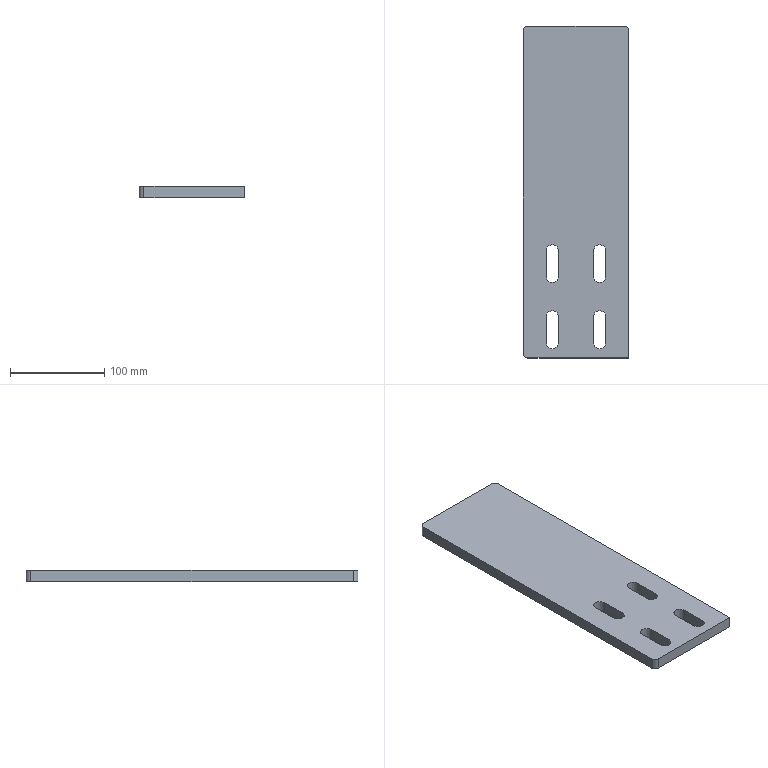Part | SolidWorks | features Extrusion 1, Fillet 1 | 1 solid | 25 faces | box 112 x 352 x 12 mm | volume 449676 mm3 | plane 14 | cylinder 11 | commonest cylinder face diameters 13 x8 10 x3
STEP:
#1=CARTESIAN_POINT('',(-56.,171.,12.));
#2=VERTEX_POINT('',#1);
#3=CARTESIAN_POINT('',(-56.,-171.,12.));
#4=VERTEX_POINT('',#3);
#5=CARTESIAN_POINT('',(-56.,176.,12.));
#6=DIRECTION('',(0.,-1.,0.));
#7=VECTOR('',#6,1000.);
#8=LINE('',#5,#7);
#9=EDGE_CURVE('',#2,#4,#8,.T.);
#10=ORIENTED_EDGE('',*,*,#9,.T.);
#11=CARTESIAN_POINT('',(-51.,-176.,12.));
#12=VERTEX_POINT('',#11);
#13=CARTESIAN_POINT('',(-51.,-171.,12.));
#14=DIRECTION('',(0.,0.,1.));
#15=DIRECTION('',(1.,0.,0.));
#16=AXIS2_PLACEMENT_3D('',#13,#14,#15);
#17=CIRCLE('',#16,5.);
#18=EDGE_CURVE('',#4,#12,#17,.T.);
#19=ORIENTED_EDGE('',*,*,#18,.T.);
#20=CARTESIAN_POINT('',(56.,-176.,12.));
#21=VERTEX_POINT('',#20);
#22=CARTESIAN_POINT('',(-56.,-176.,12.));
#23=DIRECTION('',(1.,0.,0.));
#24=VECTOR('',#23,1000.);
#25=LINE('',#22,#24);
#26=EDGE_CURVE('',#12,#21,#25,.T.);
#27=ORIENTED_EDGE('',*,*,#26,.T.);
#28=CARTESIAN_POINT('',(56.,171.,12.));
#29=VERTEX_POINT('',#28);
#30=CARTESIAN_POINT('',(56.,176.,12.));
#31=DIRECTION('',(0.,1.,0.));
#32=VECTOR('',#31,1000.);
#33=LINE('',#30,#32);
#34=EDGE_CURVE('',#21,#29,#33,.T.);
#35=ORIENTED_EDGE('',*,*,#34,.T.);
#36=CARTESIAN_POINT('',(51.,176.,12.));
#37=VERTEX_POINT('',#36);
#38=CARTESIAN_POINT('',(51.,171.,12.));
#39=DIRECTION('',(0.,0.,1.));
#40=DIRECTION('',(1.,0.,0.));
#41=AXIS2_PLACEMENT_3D('',#38,#39,#40);
#42=CIRCLE('',#41,5.);
#43=EDGE_CURVE('',#29,#37,#42,.T.);
#44=ORIENTED_EDGE('',*,*,#43,.T.);
#45=CARTESIAN_POINT('',(-51.,176.,12.));
#46=VERTEX_POINT('',#45);
#47=CARTESIAN_POINT('',(-56.,176.,12.));
#48=DIRECTION('',(-1.,0.,0.));
#49=VECTOR('',#48,1000.);
#50=LINE('',#47,#49);
#51=EDGE_CURVE('',#37,#46,#50,.T.);
#52=ORIENTED_EDGE('',*,*,#51,.T.);
#53=CARTESIAN_POINT('',(-51.,171.,12.));
#54=DIRECTION('',(0.,0.,1.));
#55=DIRECTION('',(1.,0.,0.));
#56=AXIS2_PLACEMENT_3D('',#53,#54,#55);
#57=CIRCLE('',#56,5.);
#58=EDGE_CURVE('',#46,#2,#57,.T.);
#59=ORIENTED_EDGE('',*,*,#58,.T.);
#60=EDGE_LOOP('',(#10,#19,#27,#35,#44,#52,#59));
#61=FACE_OUTER_BOUND('',#60,.T.);
#62=CARTESIAN_POINT('',(-31.5,-62.5,12.));
#63=VERTEX_POINT('',#62);
#64=CARTESIAN_POINT('',(-31.5,-89.5,12.));
#65=VERTEX_POINT('',#64);
#66=CARTESIAN_POINT('',(-31.5,-62.5,12.));
#67=DIRECTION('',(0.,-1.,0.));
#68=VECTOR('',#67,1000.);
#69=LINE('',#66,#68);
#70=EDGE_CURVE('',#63,#65,#69,.T.);
#71=ORIENTED_EDGE('',*,*,#70,.F.);
#72=CARTESIAN_POINT('',(-18.5,-62.5,12.));
#73=VERTEX_POINT('',#72);
#74=CARTESIAN_POINT('',(-25.,-62.5,12.));
#75=DIRECTION('',(0.,0.,1.));
#76=DIRECTION('',(1.,0.,0.));
#77=AXIS2_PLACEMENT_3D('',#74,#75,#76);
#78=CIRCLE('',#77,6.5);
#79=EDGE_CURVE('',#73,#63,#78,.T.);
#80=ORIENTED_EDGE('',*,*,#79,.F.);
#81=CARTESIAN_POINT('',(-18.5,-89.5,12.));
#82=VERTEX_POINT('',#81);
#83=CARTESIAN_POINT('',(-18.5,-62.5,12.));
#84=DIRECTION('',(0.,1.,0.));
#85=VECTOR('',#84,1000.);
#86=LINE('',#83,#85);
#87=EDGE_CURVE('',#82,#73,#86,.T.);
#88=ORIENTED_EDGE('',*,*,#87,.F.);
#89=CARTESIAN_POINT('',(-25.,-89.5,12.));
#90=DIRECTION('',(0.,0.,1.));
#91=DIRECTION('',(1.,0.,0.));
#92=AXIS2_PLACEMENT_3D('',#89,#90,#91);
#93=CIRCLE('',#92,6.5);
#94=EDGE_CURVE('',#65,#82,#93,.T.);
#95=ORIENTED_EDGE('',*,*,#94,.F.);
#96=EDGE_LOOP('',(#71,#80,#88,#95));
#97=FACE_BOUND('',#96,.T.);
#98=CARTESIAN_POINT('',(18.5,-62.5,12.));
#99=VERTEX_POINT('',#98);
#100=CARTESIAN_POINT('',(18.5,-89.5,12.));
#101=VERTEX_POINT('',#100);
#102=CARTESIAN_POINT('',(18.5,-62.5,12.));
#103=DIRECTION('',(0.,-1.,0.));
#104=VECTOR('',#103,1000.);
#105=LINE('',#102,#104);
#106=EDGE_CURVE('',#99,#101,#105,.T.);
#107=ORIENTED_EDGE('',*,*,#106,.F.);
#108=CARTESIAN_POINT('',(31.5,-62.5,12.));
#109=VERTEX_POINT('',#108);
#110=CARTESIAN_POINT('',(25.,-62.5,12.));
#111=DIRECTION('',(0.,0.,1.));
#112=DIRECTION('',(1.,0.,0.));
#113=AXIS2_PLACEMENT_3D('',#110,#111,#112);
#114=CIRCLE('',#113,6.5);
#115=EDGE_CURVE('',#109,#99,#114,.T.);
#116=ORIENTED_EDGE('',*,*,#115,.F.);
#117=CARTESIAN_POINT('',(31.5,-89.5,12.));
#118=VERTEX_POINT('',#117);
#119=CARTESIAN_POINT('',(31.5,-62.5,12.));
#120=DIRECTION('',(0.,1.,0.));
#121=VECTOR('',#120,1000.);
#122=LINE('',#119,#121);
#123=EDGE_CURVE('',#118,#109,#122,.T.);
#124=ORIENTED_EDGE('',*,*,#123,.F.);
#125=CARTESIAN_POINT('',(25.,-89.5,12.));
#126=DIRECTION('',(0.,0.,1.));
#127=DIRECTION('',(1.,0.,0.));
#128=AXIS2_PLACEMENT_3D('',#125,#126,#127);
#129=CIRCLE('',#128,6.5);
#130=EDGE_CURVE('',#101,#118,#129,.T.);
#131=ORIENTED_EDGE('',*,*,#130,.F.);
#132=EDGE_LOOP('',(#107,#116,#124,#131));
#133=FACE_BOUND('',#132,.T.);
#134=CARTESIAN_POINT('',(-31.5,-132.5,12.));
#135=VERTEX_POINT('',#134);
#136=CARTESIAN_POINT('',(-31.5,-159.5,12.));
#137=VERTEX_POINT('',#136);
#138=CARTESIAN_POINT('',(-31.5,-132.5,12.));
#139=DIRECTION('',(0.,-1.,0.));
#140=VECTOR('',#139,1000.);
#141=LINE('',#138,#140);
#142=EDGE_CURVE('',#135,#137,#141,.T.);
#143=ORIENTED_EDGE('',*,*,#142,.F.);
#144=CARTESIAN_POINT('',(-18.5,-132.5,12.));
#145=VERTEX_POINT('',#144);
#146=CARTESIAN_POINT('',(-25.,-132.5,12.));
#147=DIRECTION('',(0.,0.,1.));
#148=DIRECTION('',(1.,0.,0.));
#149=AXIS2_PLACEMENT_3D('',#146,#147,#148);
#150=CIRCLE('',#149,6.5);
#151=EDGE_CURVE('',#145,#135,#150,.T.);
#152=ORIENTED_EDGE('',*,*,#151,.F.);
#153=CARTESIAN_POINT('',(-18.5,-159.5,12.));
#154=VERTEX_POINT('',#153);
#155=CARTESIAN_POINT('',(-18.5,-132.5,12.));
#156=DIRECTION('',(0.,1.,0.));
#157=VECTOR('',#156,1000.);
#158=LINE('',#155,#157);
#159=EDGE_CURVE('',#154,#145,#158,.T.);
#160=ORIENTED_EDGE('',*,*,#159,.F.);
#161=CARTESIAN_POINT('',(-25.,-159.5,12.));
#162=DIRECTION('',(0.,0.,1.));
#163=DIRECTION('',(1.,0.,0.));
#164=AXIS2_PLACEMENT_3D('',#161,#162,#163);
#165=CIRCLE('',#164,6.5);
#166=EDGE_CURVE('',#137,#154,#165,.T.);
#167=ORIENTED_EDGE('',*,*,#166,.F.);
#168=EDGE_LOOP('',(#143,#152,#160,#167));
#169=FACE_BOUND('',#168,.T.);
#170=CARTESIAN_POINT('',(18.5,-132.5,12.));
#171=VERTEX_POINT('',#170);
#172=CARTESIAN_POINT('',(18.5,-159.5,12.));
#173=VERTEX_POINT('',#172);
#174=CARTESIAN_POINT('',(18.5,-132.5,12.));
#175=DIRECTION('',(0.,-1.,0.));
#176=VECTOR('',#175,1000.);
#177=LINE('',#174,#176);
#178=EDGE_CURVE('',#171,#173,#177,.T.);
#179=ORIENTED_EDGE('',*,*,#178,.F.);
#180=CARTESIAN_POINT('',(31.5,-132.5,12.));
#181=VERTEX_POINT('',#180);
#182=CARTESIAN_POINT('',(25.,-132.5,12.));
#183=DIRECTION('',(0.,0.,1.));
#184=DIRECTION('',(1.,0.,0.));
#185=AXIS2_PLACEMENT_3D('',#182,#183,#184);
#186=CIRCLE('',#185,6.5);
#187=EDGE_CURVE('',#181,#171,#186,.T.);
#188=ORIENTED_EDGE('',*,*,#187,.F.);
#189=CARTESIAN_POINT('',(31.5,-159.5,12.));
#190=VERTEX_POINT('',#189);
#191=CARTESIAN_POINT('',(31.5,-132.5,12.));
#192=DIRECTION('',(0.,1.,0.));
#193=VECTOR('',#192,1000.);
#194=LINE('',#191,#193);
#195=EDGE_CURVE('',#190,#181,#194,.T.);
#196=ORIENTED_EDGE('',*,*,#195,.F.);
#197=CARTESIAN_POINT('',(25.,-159.5,12.));
#198=DIRECTION('',(0.,0.,1.));
#199=DIRECTION('',(1.,0.,0.));
#200=AXIS2_PLACEMENT_3D('',#197,#198,#199);
#201=CIRCLE('',#200,6.5);
#202=EDGE_CURVE('',#173,#190,#201,.T.);
#203=ORIENTED_EDGE('',*,*,#202,.F.);
#204=EDGE_LOOP('',(#179,#188,#196,#203));
#205=FACE_BOUND('',#204,.T.);
#206=CARTESIAN_POINT('',(0.,0.,12.));
#207=DIRECTION('',(0.,0.,1.));
#208=DIRECTION('',(1.,0.,0.));
#209=AXIS2_PLACEMENT_3D('',#206,#207,#208);
#210=PLANE('',#209);
#211=ADVANCED_FACE('',(#61,#97,#133,#169,#205),#210,.T.);
#212=CARTESIAN_POINT('',(-18.5,-132.5,0.));
#213=VERTEX_POINT('',#212);
#214=CARTESIAN_POINT('',(-31.5,-132.5,0.));
#215=VERTEX_POINT('',#214);
#216=CARTESIAN_POINT('',(-25.,-132.5,0.));
#217=DIRECTION('',(0.,0.,1.));
#218=DIRECTION('',(1.,0.,0.));
#219=AXIS2_PLACEMENT_3D('',#216,#217,#218);
#220=CIRCLE('',#219,6.5);
#221=EDGE_CURVE('',#213,#215,#220,.T.);
#222=ORIENTED_EDGE('',*,*,#221,.T.);
#223=CARTESIAN_POINT('',(-31.5,-159.5,0.));
#224=VERTEX_POINT('',#223);
#225=CARTESIAN_POINT('',(-31.5,-132.5,0.));
#226=DIRECTION('',(0.,-1.,0.));
#227=VECTOR('',#226,1000.);
#228=LINE('',#225,#227);
#229=EDGE_CURVE('',#215,#224,#228,.T.);
#230=ORIENTED_EDGE('',*,*,#229,.T.);
#231=CARTESIAN_POINT('',(-18.5,-159.5,0.));
#232=VERTEX_POINT('',#231);
#233=CARTESIAN_POINT('',(-25.,-159.5,0.));
#234=DIRECTION('',(0.,0.,1.));
#235=DIRECTION('',(1.,0.,0.));
#236=AXIS2_PLACEMENT_3D('',#233,#234,#235);
#237=CIRCLE('',#236,6.5);
#238=EDGE_CURVE('',#224,#232,#237,.T.);
#239=ORIENTED_EDGE('',*,*,#238,.T.);
#240=CARTESIAN_POINT('',(-18.5,-132.5,0.));
#241=DIRECTION('',(0.,1.,0.));
#242=VECTOR('',#241,1000.);
#243=LINE('',#240,#242);
#244=EDGE_CURVE('',#232,#213,#243,.T.);
#245=ORIENTED_EDGE('',*,*,#244,.T.);
#246=EDGE_LOOP('',(#222,#230,#239,#245));
#247=FACE_BOUND('',#246,.T.);
#248=CARTESIAN_POINT('',(-18.5,-62.5,0.));
#249=VERTEX_POINT('',#248);
#250=CARTESIAN_POINT('',(-31.5,-62.5,0.));
#251=VERTEX_POINT('',#250);
#252=CARTESIAN_POINT('',(-25.,-62.5,0.));
#253=DIRECTION('',(0.,0.,1.));
#254=DIRECTION('',(1.,0.,0.));
#255=AXIS2_PLACEMENT_3D('',#252,#253,#254);
#256=CIRCLE('',#255,6.5);
#257=EDGE_CURVE('',#249,#251,#256,.T.);
#258=ORIENTED_EDGE('',*,*,#257,.T.);
#259=CARTESIAN_POINT('',(-31.5,-89.5,0.));
#260=VERTEX_POINT('',#259);
#261=CARTESIAN_POINT('',(-31.5,-62.5,0.));
#262=DIRECTION('',(0.,-1.,0.));
#263=VECTOR('',#262,1000.);
#264=LINE('',#261,#263);
#265=EDGE_CURVE('',#251,#260,#264,.T.);
#266=ORIENTED_EDGE('',*,*,#265,.T.);
#267=CARTESIAN_POINT('',(-18.5,-89.5,0.));
#268=VERTEX_POINT('',#267);
#269=CARTESIAN_POINT('',(-25.,-89.5,0.));
#270=DIRECTION('',(0.,0.,1.));
#271=DIRECTION('',(1.,0.,0.));
#272=AXIS2_PLACEMENT_3D('',#269,#270,#271);
#273=CIRCLE('',#272,6.5);
#274=EDGE_CURVE('',#260,#268,#273,.T.);
#275=ORIENTED_EDGE('',*,*,#274,.T.);
#276=CARTESIAN_POINT('',(-18.5,-62.5,0.));
#277=DIRECTION('',(0.,1.,0.));
#278=VECTOR('',#277,1000.);
#279=LINE('',#276,#278);
#280=EDGE_CURVE('',#268,#249,#279,.T.);
#281=ORIENTED_EDGE('',*,*,#280,.T.);
#282=EDGE_LOOP('',(#258,#266,#275,#281));
#283=FACE_BOUND('',#282,.T.);
#284=CARTESIAN_POINT('',(-51.,-176.,0.));
#285=VERTEX_POINT('',#284);
#286=CARTESIAN_POINT('',(56.,-176.,0.));
#287=VERTEX_POINT('',#286);
#288=CARTESIAN_POINT('',(-56.,-176.,0.));
#289=DIRECTION('',(1.,0.,0.));
#290=VECTOR('',#289,1000.);
#291=LINE('',#288,#290);
#292=EDGE_CURVE('',#285,#287,#291,.T.);
#293=ORIENTED_EDGE('',*,*,#292,.F.);
#294=CARTESIAN_POINT('',(-56.,-171.,0.));
#295=VERTEX_POINT('',#294);
#296=CARTESIAN_POINT('',(-51.,-171.,0.));
#297=DIRECTION('',(0.,0.,-1.));
#298=DIRECTION('',(1.,0.,0.));
#299=AXIS2_PLACEMENT_3D('',#296,#297,#298);
#300=CIRCLE('',#299,5.);
#301=EDGE_CURVE('',#285,#295,#300,.T.);
#302=ORIENTED_EDGE('',*,*,#301,.T.);
#303=CARTESIAN_POINT('',(-56.,171.,0.));
#304=VERTEX_POINT('',#303);
#305=CARTESIAN_POINT('',(-56.,176.,0.));
#306=DIRECTION('',(0.,-1.,0.));
#307=VECTOR('',#306,1000.);
#308=LINE('',#305,#307);
#309=EDGE_CURVE('',#304,#295,#308,.T.);
#310=ORIENTED_EDGE('',*,*,#309,.F.);
#311=CARTESIAN_POINT('',(-51.,176.,0.));
#312=VERTEX_POINT('',#311);
#313=CARTESIAN_POINT('',(-51.,171.,0.));
#314=DIRECTION('',(0.,0.,-1.));
#315=DIRECTION('',(1.,0.,0.));
#316=AXIS2_PLACEMENT_3D('',#313,#314,#315);
#317=CIRCLE('',#316,5.);
#318=EDGE_CURVE('',#304,#312,#317,.T.);
#319=ORIENTED_EDGE('',*,*,#318,.T.);
#320=CARTESIAN_POINT('',(51.,176.,0.));
#321=VERTEX_POINT('',#320);
#322=CARTESIAN_POINT('',(-56.,176.,0.));
#323=DIRECTION('',(-1.,0.,0.));
#324=VECTOR('',#323,1000.);
#325=LINE('',#322,#324);
#326=EDGE_CURVE('',#321,#312,#325,.T.);
#327=ORIENTED_EDGE('',*,*,#326,.F.);
#328=CARTESIAN_POINT('',(56.,171.,0.));
#329=VERTEX_POINT('',#328);
#330=CARTESIAN_POINT('',(51.,171.,0.));
#331=DIRECTION('',(0.,0.,-1.));
#332=DIRECTION('',(1.,0.,0.));
#333=AXIS2_PLACEMENT_3D('',#330,#331,#332);
#334=CIRCLE('',#333,5.);
#335=EDGE_CURVE('',#321,#329,#334,.T.);
#336=ORIENTED_EDGE('',*,*,#335,.T.);
#337=CARTESIAN_POINT('',(56.,176.,0.));
#338=DIRECTION('',(0.,1.,0.));
#339=VECTOR('',#338,1000.);
#340=LINE('',#337,#339);
#341=EDGE_CURVE('',#287,#329,#340,.T.);
#342=ORIENTED_EDGE('',*,*,#341,.F.);
#343=EDGE_LOOP('',(#293,#302,#310,#319,#327,#336,#342));
#344=FACE_OUTER_BOUND('',#343,.T.);
#345=CARTESIAN_POINT('',(31.5,-62.5,0.));
#346=VERTEX_POINT('',#345);
#347=CARTESIAN_POINT('',(18.5,-62.5,0.));
#348=VERTEX_POINT('',#347);
#349=CARTESIAN_POINT('',(25.,-62.5,0.));
#350=DIRECTION('',(0.,0.,1.));
#351=DIRECTION('',(1.,0.,0.));
#352=AXIS2_PLACEMENT_3D('',#349,#350,#351);
#353=CIRCLE('',#352,6.5);
#354=EDGE_CURVE('',#346,#348,#353,.T.);
#355=ORIENTED_EDGE('',*,*,#354,.T.);
#356=CARTESIAN_POINT('',(18.5,-89.5,0.));
#357=VERTEX_POINT('',#356);
#358=CARTESIAN_POINT('',(18.5,-62.5,0.));
#359=DIRECTION('',(0.,-1.,0.));
#360=VECTOR('',#359,1000.);
#361=LINE('',#358,#360);
#362=EDGE_CURVE('',#348,#357,#361,.T.);
#363=ORIENTED_EDGE('',*,*,#362,.T.);
#364=CARTESIAN_POINT('',(31.5,-89.5,0.));
#365=VERTEX_POINT('',#364);
#366=CARTESIAN_POINT('',(25.,-89.5,0.));
#367=DIRECTION('',(0.,0.,1.));
#368=DIRECTION('',(1.,0.,0.));
#369=AXIS2_PLACEMENT_3D('',#366,#367,#368);
#370=CIRCLE('',#369,6.5);
#371=EDGE_CURVE('',#357,#365,#370,.T.);
#372=ORIENTED_EDGE('',*,*,#371,.T.);
#373=CARTESIAN_POINT('',(31.5,-62.5,0.));
#374=DIRECTION('',(0.,1.,0.));
#375=VECTOR('',#374,1000.);
#376=LINE('',#373,#375);
#377=EDGE_CURVE('',#365,#346,#376,.T.);
#378=ORIENTED_EDGE('',*,*,#377,.T.);
#379=EDGE_LOOP('',(#355,#363,#372,#378));
#380=FACE_BOUND('',#379,.T.);
#381=CARTESIAN_POINT('',(31.5,-132.5,0.));
#382=VERTEX_POINT('',#381);
#383=CARTESIAN_POINT('',(18.5,-132.5,0.));
#384=VERTEX_POINT('',#383);
#385=CARTESIAN_POINT('',(25.,-132.5,0.));
#386=DIRECTION('',(0.,0.,1.));
#387=DIRECTION('',(1.,0.,0.));
#388=AXIS2_PLACEMENT_3D('',#385,#386,#387);
#389=CIRCLE('',#388,6.5);
#390=EDGE_CURVE('',#382,#384,#389,.T.);
#391=ORIENTED_EDGE('',*,*,#390,.T.);
#392=CARTESIAN_POINT('',(18.5,-159.5,0.));
#393=VERTEX_POINT('',#392);
#394=CARTESIAN_POINT('',(18.5,-132.5,0.));
#395=DIRECTION('',(0.,-1.,0.));
#396=VECTOR('',#395,1000.);
#397=LINE('',#394,#396);
#398=EDGE_CURVE('',#384,#393,#397,.T.);
#399=ORIENTED_EDGE('',*,*,#398,.T.);
#400=CARTESIAN_POINT('',(31.5,-159.5,0.));
#401=VERTEX_POINT('',#400);
#402=CARTESIAN_POINT('',(25.,-159.5,0.));
#403=DIRECTION('',(0.,0.,1.));
#404=DIRECTION('',(1.,0.,0.));
#405=AXIS2_PLACEMENT_3D('',#402,#403,#404);
#406=CIRCLE('',#405,6.5);
#407=EDGE_CURVE('',#393,#401,#406,.T.);
#408=ORIENTED_EDGE('',*,*,#407,.T.);
#409=CARTESIAN_POINT('',(31.5,-132.5,0.));
#410=DIRECTION('',(0.,1.,0.));
#411=VECTOR('',#410,1000.);
#412=LINE('',#409,#411);
#413=EDGE_CURVE('',#401,#382,#412,.T.);
#414=ORIENTED_EDGE('',*,*,#413,.T.);
#415=EDGE_LOOP('',(#391,#399,#408,#414));
#416=FACE_BOUND('',#415,.T.);
#417=CARTESIAN_POINT('',(0.,0.,0.));
#418=DIRECTION('',(0.,0.,1.));
#419=DIRECTION('',(1.,0.,0.));
#420=AXIS2_PLACEMENT_3D('',#417,#418,#419);
#421=PLANE('',#420);
#422=ADVANCED_FACE('',(#247,#283,#344,#380,#416),#421,.F.);
#423=ORIENTED_EDGE('',*,*,#341,.T.);
#424=CARTESIAN_POINT('',(56.,171.,12.));
#425=DIRECTION('',(0.,0.,1.));
#426=VECTOR('',#425,1000.);
#427=LINE('',#424,#426);
#428=EDGE_CURVE('',#329,#29,#427,.T.);
#429=ORIENTED_EDGE('',*,*,#428,.T.);
#430=ORIENTED_EDGE('',*,*,#34,.F.);
#431=CARTESIAN_POINT('',(56.,-176.,12.));
#432=DIRECTION('',(0.,0.,-1.));
#433=VECTOR('',#432,1000.);
#434=LINE('',#431,#433);
#435=EDGE_CURVE('',#21,#287,#434,.T.);
#436=ORIENTED_EDGE('',*,*,#435,.T.);
#437=EDGE_LOOP('',(#423,#429,#430,#436));
#438=FACE_OUTER_BOUND('',#437,.T.);
#439=CARTESIAN_POINT('',(56.,176.,12.));
#440=DIRECTION('',(-1.,0.,0.));
#441=DIRECTION('',(0.,-1.,0.));
#442=AXIS2_PLACEMENT_3D('',#439,#440,#441);
#443=PLANE('',#442);
#444=ADVANCED_FACE('',(#438),#443,.F.);
#445=ORIENTED_EDGE('',*,*,#51,.F.);
#446=CARTESIAN_POINT('',(51.,176.,12.));
#447=DIRECTION('',(0.,0.,-1.));
#448=VECTOR('',#447,1000.);
#449=LINE('',#446,#448);
#450=EDGE_CURVE('',#37,#321,#449,.T.);
#451=ORIENTED_EDGE('',*,*,#450,.T.);
#452=ORIENTED_EDGE('',*,*,#326,.T.);
#453=CARTESIAN_POINT('',(-51.,176.,12.));
#454=DIRECTION('',(0.,0.,1.));
#455=VECTOR('',#454,1000.);
#456=LINE('',#453,#455);
#457=EDGE_CURVE('',#312,#46,#456,.T.);
#458=ORIENTED_EDGE('',*,*,#457,.T.);
#459=EDGE_LOOP('',(#445,#451,#452,#458));
#460=FACE_OUTER_BOUND('',#459,.T.);
#461=CARTESIAN_POINT('',(-56.,176.,12.));
#462=DIRECTION('',(0.,-1.,0.));
#463=DIRECTION('',(0.,0.,-1.));
#464=AXIS2_PLACEMENT_3D('',#461,#462,#463);
#465=PLANE('',#464);
#466=ADVANCED_FACE('',(#460),#465,.F.);
#467=ORIENTED_EDGE('',*,*,#309,.T.);
#468=CARTESIAN_POINT('',(-56.,-171.,12.));
#469=DIRECTION('',(0.,0.,1.));
#470=VECTOR('',#469,1000.);
#471=LINE('',#468,#470);
#472=EDGE_CURVE('',#295,#4,#471,.T.);
#473=ORIENTED_EDGE('',*,*,#472,.T.);
#474=ORIENTED_EDGE('',*,*,#9,.F.);
#475=CARTESIAN_POINT('',(-56.,171.,12.));
#476=DIRECTION('',(0.,0.,-1.));
#477=VECTOR('',#476,1000.);
#478=LINE('',#475,#477);
#479=EDGE_CURVE('',#2,#304,#478,.T.);
#480=ORIENTED_EDGE('',*,*,#479,.T.);
#481=EDGE_LOOP('',(#467,#473,#474,#480));
#482=FACE_OUTER_BOUND('',#481,.T.);
#483=CARTESIAN_POINT('',(-56.,176.,12.));
#484=DIRECTION('',(1.,0.,0.));
#485=DIRECTION('',(0.,1.,0.));
#486=AXIS2_PLACEMENT_3D('',#483,#484,#485);
#487=PLANE('',#486);
#488=ADVANCED_FACE('',(#482),#487,.F.);
#489=ORIENTED_EDGE('',*,*,#26,.F.);
#490=CARTESIAN_POINT('',(-51.,-176.,12.));
#491=DIRECTION('',(0.,0.,-1.));
#492=VECTOR('',#491,1000.);
#493=LINE('',#490,#492);
#494=EDGE_CURVE('',#12,#285,#493,.T.);
#495=ORIENTED_EDGE('',*,*,#494,.T.);
#496=ORIENTED_EDGE('',*,*,#292,.T.);
#497=ORIENTED_EDGE('',*,*,#435,.F.);
#498=EDGE_LOOP('',(#489,#495,#496,#497));
#499=FACE_OUTER_BOUND('',#498,.T.);
#500=CARTESIAN_POINT('',(-56.,-176.,12.));
#501=DIRECTION('',(0.,1.,0.));
#502=DIRECTION('',(0.,0.,1.));
#503=AXIS2_PLACEMENT_3D('',#500,#501,#502);
#504=PLANE('',#503);
#505=ADVANCED_FACE('',(#499),#504,.F.);
#506=ORIENTED_EDGE('',*,*,#257,.F.);
#507=CARTESIAN_POINT('',(-18.5,-62.5,12.));
#508=DIRECTION('',(0.,0.,-1.));
#509=VECTOR('',#508,1000.);
#510=LINE('',#507,#509);
#511=EDGE_CURVE('',#73,#249,#510,.T.);
#512=ORIENTED_EDGE('',*,*,#511,.F.);
#513=ORIENTED_EDGE('',*,*,#79,.T.);
#514=CARTESIAN_POINT('',(-31.5,-62.5,12.));
#515=DIRECTION('',(0.,0.,-1.));
#516=VECTOR('',#515,1000.);
#517=LINE('',#514,#516);
#518=EDGE_CURVE('',#63,#251,#517,.T.);
#519=ORIENTED_EDGE('',*,*,#518,.T.);
#520=EDGE_LOOP('',(#506,#512,#513,#519));
#521=FACE_OUTER_BOUND('',#520,.T.);
#522=CARTESIAN_POINT('',(-25.,-62.5,12.));
#523=DIRECTION('',(0.,0.,-1.));
#524=DIRECTION('',(-1.,0.,0.));
#525=AXIS2_PLACEMENT_3D('',#522,#523,#524);
#526=CYLINDRICAL_SURFACE('',#525,6.5);
#527=ADVANCED_FACE('',(#521),#526,.F.);
#528=ORIENTED_EDGE('',*,*,#265,.F.);
#529=ORIENTED_EDGE('',*,*,#518,.F.);
#530=ORIENTED_EDGE('',*,*,#70,.T.);
#531=CARTESIAN_POINT('',(-31.5,-89.5,12.));
#532=DIRECTION('',(0.,0.,-1.));
#533=VECTOR('',#532,1000.);
#534=LINE('',#531,#533);
#535=EDGE_CURVE('',#65,#260,#534,.T.);
#536=ORIENTED_EDGE('',*,*,#535,.T.);
#537=EDGE_LOOP('',(#528,#529,#530,#536));
#538=FACE_OUTER_BOUND('',#537,.T.);
#539=CARTESIAN_POINT('',(-31.5,-62.5,12.));
#540=DIRECTION('',(1.,0.,0.));
#541=DIRECTION('',(0.,1.,0.));
#542=AXIS2_PLACEMENT_3D('',#539,#540,#541);
#543=PLANE('',#542);
#544=ADVANCED_FACE('',(#538),#543,.T.);
#545=ORIENTED_EDGE('',*,*,#274,.F.);
#546=ORIENTED_EDGE('',*,*,#535,.F.);
#547=ORIENTED_EDGE('',*,*,#94,.T.);
#548=CARTESIAN_POINT('',(-18.5,-89.5,12.));
#549=DIRECTION('',(0.,0.,-1.));
#550=VECTOR('',#549,1000.);
#551=LINE('',#548,#550);
#552=EDGE_CURVE('',#82,#268,#551,.T.);
#553=ORIENTED_EDGE('',*,*,#552,.T.);
#554=EDGE_LOOP('',(#545,#546,#547,#553));
#555=FACE_OUTER_BOUND('',#554,.T.);
#556=CARTESIAN_POINT('',(-25.,-89.5,12.));
#557=DIRECTION('',(0.,0.,-1.));
#558=DIRECTION('',(-1.,0.,0.));
#559=AXIS2_PLACEMENT_3D('',#556,#557,#558);
#560=CYLINDRICAL_SURFACE('',#559,6.5);
#561=ADVANCED_FACE('',(#555),#560,.F.);
#562=ORIENTED_EDGE('',*,*,#280,.F.);
#563=ORIENTED_EDGE('',*,*,#552,.F.);
#564=ORIENTED_EDGE('',*,*,#87,.T.);
#565=ORIENTED_EDGE('',*,*,#511,.T.);
#566=EDGE_LOOP('',(#562,#563,#564,#565));
#567=FACE_OUTER_BOUND('',#566,.T.);
#568=CARTESIAN_POINT('',(-18.5,-62.5,12.));
#569=DIRECTION('',(-1.,0.,0.));
#570=DIRECTION('',(0.,0.,1.));
#571=AXIS2_PLACEMENT_3D('',#568,#569,#570);
#572=PLANE('',#571);
#573=ADVANCED_FACE('',(#567),#572,.T.);
#574=ORIENTED_EDGE('',*,*,#354,.F.);
#575=CARTESIAN_POINT('',(31.5,-62.5,12.));
#576=DIRECTION('',(0.,0.,-1.));
#577=VECTOR('',#576,1000.);
#578=LINE('',#575,#577);
#579=EDGE_CURVE('',#109,#346,#578,.T.);
#580=ORIENTED_EDGE('',*,*,#579,.F.);
#581=ORIENTED_EDGE('',*,*,#115,.T.);
#582=CARTESIAN_POINT('',(18.5,-62.5,12.));
#583=DIRECTION('',(0.,0.,-1.));
#584=VECTOR('',#583,1000.);
#585=LINE('',#582,#584);
#586=EDGE_CURVE('',#99,#348,#585,.T.);
#587=ORIENTED_EDGE('',*,*,#586,.T.);
#588=EDGE_LOOP('',(#574,#580,#581,#587));
#589=FACE_OUTER_BOUND('',#588,.T.);
#590=CARTESIAN_POINT('',(25.,-62.5,12.));
#591=DIRECTION('',(0.,0.,-1.));
#592=DIRECTION('',(-1.,0.,0.));
#593=AXIS2_PLACEMENT_3D('',#590,#591,#592);
#594=CYLINDRICAL_SURFACE('',#593,6.5);
#595=ADVANCED_FACE('',(#589),#594,.F.);
#596=ORIENTED_EDGE('',*,*,#362,.F.);
#597=ORIENTED_EDGE('',*,*,#586,.F.);
#598=ORIENTED_EDGE('',*,*,#106,.T.);
#599=CARTESIAN_POINT('',(18.5,-89.5,12.));
#600=DIRECTION('',(0.,0.,-1.));
#601=VECTOR('',#600,1000.);
#602=LINE('',#599,#601);
#603=EDGE_CURVE('',#101,#357,#602,.T.);
#604=ORIENTED_EDGE('',*,*,#603,.T.);
#605=EDGE_LOOP('',(#596,#597,#598,#604));
#606=FACE_OUTER_BOUND('',#605,.T.);
#607=CARTESIAN_POINT('',(18.5,-62.5,12.));
#608=DIRECTION('',(1.,0.,0.));
#609=DIRECTION('',(0.,0.,-1.));
#610=AXIS2_PLACEMENT_3D('',#607,#608,#609);
#611=PLANE('',#610);
#612=ADVANCED_FACE('',(#606),#611,.T.);
#613=ORIENTED_EDGE('',*,*,#371,.F.);
#614=ORIENTED_EDGE('',*,*,#603,.F.);
#615=ORIENTED_EDGE('',*,*,#130,.T.);
#616=CARTESIAN_POINT('',(31.5,-89.5,12.));
#617=DIRECTION('',(0.,0.,-1.));
#618=VECTOR('',#617,1000.);
#619=LINE('',#616,#618);
#620=EDGE_CURVE('',#118,#365,#619,.T.);
#621=ORIENTED_EDGE('',*,*,#620,.T.);
#622=EDGE_LOOP('',(#613,#614,#615,#621));
#623=FACE_OUTER_BOUND('',#622,.T.);
#624=CARTESIAN_POINT('',(25.,-89.5,12.));
#625=DIRECTION('',(0.,0.,-1.));
#626=DIRECTION('',(-1.,0.,0.));
#627=AXIS2_PLACEMENT_3D('',#624,#625,#626);
#628=CYLINDRICAL_SURFACE('',#627,6.5);
#629=ADVANCED_FACE('',(#623),#628,.F.);
#630=ORIENTED_EDGE('',*,*,#377,.F.);
#631=ORIENTED_EDGE('',*,*,#620,.F.);
#632=ORIENTED_EDGE('',*,*,#123,.T.);
#633=ORIENTED_EDGE('',*,*,#579,.T.);
#634=EDGE_LOOP('',(#630,#631,#632,#633));
#635=FACE_OUTER_BOUND('',#634,.T.);
#636=CARTESIAN_POINT('',(31.5,-62.5,12.));
#637=DIRECTION('',(-1.,0.,0.));
#638=DIRECTION('',(0.,0.,1.));
#639=AXIS2_PLACEMENT_3D('',#636,#637,#638);
#640=PLANE('',#639);
#641=ADVANCED_FACE('',(#635),#640,.T.);
#642=ORIENTED_EDGE('',*,*,#221,.F.);
#643=CARTESIAN_POINT('',(-18.5,-132.5,12.));
#644=DIRECTION('',(0.,0.,-1.));
#645=VECTOR('',#644,1000.);
#646=LINE('',#643,#645);
#647=EDGE_CURVE('',#145,#213,#646,.T.);
#648=ORIENTED_EDGE('',*,*,#647,.F.);
#649=ORIENTED_EDGE('',*,*,#151,.T.);
#650=CARTESIAN_POINT('',(-31.5,-132.5,12.));
#651=DIRECTION('',(0.,0.,-1.));
#652=VECTOR('',#651,1000.);
#653=LINE('',#650,#652);
#654=EDGE_CURVE('',#135,#215,#653,.T.);
#655=ORIENTED_EDGE('',*,*,#654,.T.);
#656=EDGE_LOOP('',(#642,#648,#649,#655));
#657=FACE_OUTER_BOUND('',#656,.T.);
#658=CARTESIAN_POINT('',(-25.,-132.5,12.));
#659=DIRECTION('',(0.,0.,-1.));
#660=DIRECTION('',(-1.,0.,0.));
#661=AXIS2_PLACEMENT_3D('',#658,#659,#660);
#662=CYLINDRICAL_SURFACE('',#661,6.5);
#663=ADVANCED_FACE('',(#657),#662,.F.);
#664=ORIENTED_EDGE('',*,*,#229,.F.);
#665=ORIENTED_EDGE('',*,*,#654,.F.);
#666=ORIENTED_EDGE('',*,*,#142,.T.);
#667=CARTESIAN_POINT('',(-31.5,-159.5,12.));
#668=DIRECTION('',(0.,0.,-1.));
#669=VECTOR('',#668,1000.);
#670=LINE('',#667,#669);
#671=EDGE_CURVE('',#137,#224,#670,.T.);
#672=ORIENTED_EDGE('',*,*,#671,.T.);
#673=EDGE_LOOP('',(#664,#665,#666,#672));
#674=FACE_OUTER_BOUND('',#673,.T.);
#675=CARTESIAN_POINT('',(-31.5,-132.5,12.));
#676=DIRECTION('',(1.,0.,0.));
#677=DIRECTION('',(0.,1.,0.));
#678=AXIS2_PLACEMENT_3D('',#675,#676,#677);
#679=PLANE('',#678);
#680=ADVANCED_FACE('',(#674),#679,.T.);
#681=ORIENTED_EDGE('',*,*,#238,.F.);
#682=ORIENTED_EDGE('',*,*,#671,.F.);
#683=ORIENTED_EDGE('',*,*,#166,.T.);
#684=CARTESIAN_POINT('',(-18.5,-159.5,12.));
#685=DIRECTION('',(0.,0.,-1.));
#686=VECTOR('',#685,1000.);
#687=LINE('',#684,#686);
#688=EDGE_CURVE('',#154,#232,#687,.T.);
#689=ORIENTED_EDGE('',*,*,#688,.T.);
#690=EDGE_LOOP('',(#681,#682,#683,#689));
#691=FACE_OUTER_BOUND('',#690,.T.);
#692=CARTESIAN_POINT('',(-25.,-159.5,12.));
#693=DIRECTION('',(0.,0.,-1.));
#694=DIRECTION('',(-1.,0.,0.));
#695=AXIS2_PLACEMENT_3D('',#692,#693,#694);
#696=CYLINDRICAL_SURFACE('',#695,6.5);
#697=ADVANCED_FACE('',(#691),#696,.F.);
#698=ORIENTED_EDGE('',*,*,#244,.F.);
#699=ORIENTED_EDGE('',*,*,#688,.F.);
#700=ORIENTED_EDGE('',*,*,#159,.T.);
#701=ORIENTED_EDGE('',*,*,#647,.T.);
#702=EDGE_LOOP('',(#698,#699,#700,#701));
#703=FACE_OUTER_BOUND('',#702,.T.);
#704=CARTESIAN_POINT('',(-18.5,-132.5,12.));
#705=DIRECTION('',(-1.,0.,0.));
#706=DIRECTION('',(0.,-1.,0.));
#707=AXIS2_PLACEMENT_3D('',#704,#705,#706);
#708=PLANE('',#707);
#709=ADVANCED_FACE('',(#703),#708,.T.);
#710=ORIENTED_EDGE('',*,*,#390,.F.);
#711=CARTESIAN_POINT('',(31.5,-132.5,12.));
#712=DIRECTION('',(0.,0.,-1.));
#713=VECTOR('',#712,1000.);
#714=LINE('',#711,#713);
#715=EDGE_CURVE('',#181,#382,#714,.T.);
#716=ORIENTED_EDGE('',*,*,#715,.F.);
#717=ORIENTED_EDGE('',*,*,#187,.T.);
#718=CARTESIAN_POINT('',(18.5,-132.5,12.));
#719=DIRECTION('',(0.,0.,-1.));
#720=VECTOR('',#719,1000.);
#721=LINE('',#718,#720);
#722=EDGE_CURVE('',#171,#384,#721,.T.);
#723=ORIENTED_EDGE('',*,*,#722,.T.);
#724=EDGE_LOOP('',(#710,#716,#717,#723));
#725=FACE_OUTER_BOUND('',#724,.T.);
#726=CARTESIAN_POINT('',(25.,-132.5,12.));
#727=DIRECTION('',(0.,0.,-1.));
#728=DIRECTION('',(-1.,0.,0.));
#729=AXIS2_PLACEMENT_3D('',#726,#727,#728);
#730=CYLINDRICAL_SURFACE('',#729,6.5);
#731=ADVANCED_FACE('',(#725),#730,.F.);
#732=ORIENTED_EDGE('',*,*,#398,.F.);
#733=ORIENTED_EDGE('',*,*,#722,.F.);
#734=ORIENTED_EDGE('',*,*,#178,.T.);
#735=CARTESIAN_POINT('',(18.5,-159.5,12.));
#736=DIRECTION('',(0.,0.,-1.));
#737=VECTOR('',#736,1000.);
#738=LINE('',#735,#737);
#739=EDGE_CURVE('',#173,#393,#738,.T.);
#740=ORIENTED_EDGE('',*,*,#739,.T.);
#741=EDGE_LOOP('',(#732,#733,#734,#740));
#742=FACE_OUTER_BOUND('',#741,.T.);
#743=CARTESIAN_POINT('',(18.5,-132.5,12.));
#744=DIRECTION('',(1.,0.,0.));
#745=DIRECTION('',(0.,0.,-1.));
#746=AXIS2_PLACEMENT_3D('',#743,#744,#745);
#747=PLANE('',#746);
#748=ADVANCED_FACE('',(#742),#747,.T.);
#749=ORIENTED_EDGE('',*,*,#407,.F.);
#750=ORIENTED_EDGE('',*,*,#739,.F.);
#751=ORIENTED_EDGE('',*,*,#202,.T.);
#752=CARTESIAN_POINT('',(31.5,-159.5,12.));
#753=DIRECTION('',(0.,0.,-1.));
#754=VECTOR('',#753,1000.);
#755=LINE('',#752,#754);
#756=EDGE_CURVE('',#190,#401,#755,.T.);
#757=ORIENTED_EDGE('',*,*,#756,.T.);
#758=EDGE_LOOP('',(#749,#750,#751,#757));
#759=FACE_OUTER_BOUND('',#758,.T.);
#760=CARTESIAN_POINT('',(25.,-159.5,12.));
#761=DIRECTION('',(0.,0.,-1.));
#762=DIRECTION('',(-1.,0.,0.));
#763=AXIS2_PLACEMENT_3D('',#760,#761,#762);
#764=CYLINDRICAL_SURFACE('',#763,6.5);
#765=ADVANCED_FACE('',(#759),#764,.F.);
#766=ORIENTED_EDGE('',*,*,#413,.F.);
#767=ORIENTED_EDGE('',*,*,#756,.F.);
#768=ORIENTED_EDGE('',*,*,#195,.T.);
#769=ORIENTED_EDGE('',*,*,#715,.T.);
#770=EDGE_LOOP('',(#766,#767,#768,#769));
#771=FACE_OUTER_BOUND('',#770,.T.);
#772=CARTESIAN_POINT('',(31.5,-132.5,12.));
#773=DIRECTION('',(-1.,0.,0.));
#774=DIRECTION('',(0.,0.,1.));
#775=AXIS2_PLACEMENT_3D('',#772,#773,#774);
#776=PLANE('',#775);
#777=ADVANCED_FACE('',(#771),#776,.T.);
#778=ORIENTED_EDGE('',*,*,#18,.F.);
#779=ORIENTED_EDGE('',*,*,#472,.F.);
#780=ORIENTED_EDGE('',*,*,#301,.F.);
#781=ORIENTED_EDGE('',*,*,#494,.F.);
#782=EDGE_LOOP('',(#778,#779,#780,#781));
#783=FACE_OUTER_BOUND('',#782,.T.);
#784=CARTESIAN_POINT('',(-51.,-171.,12.));
#785=DIRECTION('',(0.,0.,-1.));
#786=DIRECTION('',(-1.,0.,0.));
#787=AXIS2_PLACEMENT_3D('',#784,#785,#786);
#788=CYLINDRICAL_SURFACE('',#787,5.);
#789=ADVANCED_FACE('',(#783),#788,.T.);
#790=ORIENTED_EDGE('',*,*,#43,.F.);
#791=ORIENTED_EDGE('',*,*,#428,.F.);
#792=ORIENTED_EDGE('',*,*,#335,.F.);
#793=ORIENTED_EDGE('',*,*,#450,.F.);
#794=EDGE_LOOP('',(#790,#791,#792,#793));
#795=FACE_OUTER_BOUND('',#794,.T.);
#796=CARTESIAN_POINT('',(51.,171.,12.));
#797=DIRECTION('',(0.,0.,-1.));
#798=DIRECTION('',(-1.,0.,0.));
#799=AXIS2_PLACEMENT_3D('',#796,#797,#798);
#800=CYLINDRICAL_SURFACE('',#799,5.);
#801=ADVANCED_FACE('',(#795),#800,.T.);
#802=ORIENTED_EDGE('',*,*,#58,.F.);
#803=ORIENTED_EDGE('',*,*,#457,.F.);
#804=ORIENTED_EDGE('',*,*,#318,.F.);
#805=ORIENTED_EDGE('',*,*,#479,.F.);
#806=EDGE_LOOP('',(#802,#803,#804,#805));
#807=FACE_OUTER_BOUND('',#806,.T.);
#808=CARTESIAN_POINT('',(-51.,171.,12.));
#809=DIRECTION('',(0.,0.,-1.));
#810=DIRECTION('',(-1.,0.,0.));
#811=AXIS2_PLACEMENT_3D('',#808,#809,#810);
#812=CYLINDRICAL_SURFACE('',#811,5.);
#813=ADVANCED_FACE('',(#807),#812,.T.);
#814=CLOSED_SHELL('',(#211,#422,#444,#466,#488,#505,#527,#544,#561,#573,#595,#612,#629,#641,#663,#680,#697,#709,#731,#748,#765,#777,#789,#801,#813));
#815=MANIFOLD_SOLID_BREP('',#814);
#816=CARTESIAN_POINT('',(0.,0.,0.));
#817=DIRECTION('',(0.,0.,1.));
#818=DIRECTION('',(1.,0.,0.));
#819=AXIS2_PLACEMENT_3D('',#816,#817,#818);
#820=(LENGTH_UNIT()NAMED_UNIT(*)SI_UNIT(.MILLI.,.METRE.));
#821=UNCERTAINTY_MEASURE_WITH_UNIT(LENGTH_MEASURE(0.00001),#820,'','');
#822=(NAMED_UNIT(*)PLANE_ANGLE_UNIT()SI_UNIT($,.RADIAN.));
#823=(NAMED_UNIT(*)SI_UNIT($,.STERADIAN.)SOLID_ANGLE_UNIT());
#824=(GEOMETRIC_REPRESENTATION_CONTEXT(3)GLOBAL_UNCERTAINTY_ASSIGNED_CONTEXT((#821))GLOBAL_UNIT_ASSIGNED_CONTEXT((#820,#822,#823))REPRESENTATION_CONTEXT('',''));
#825=ADVANCED_BREP_SHAPE_REPRESENTATION('',(#815,#819),#824);